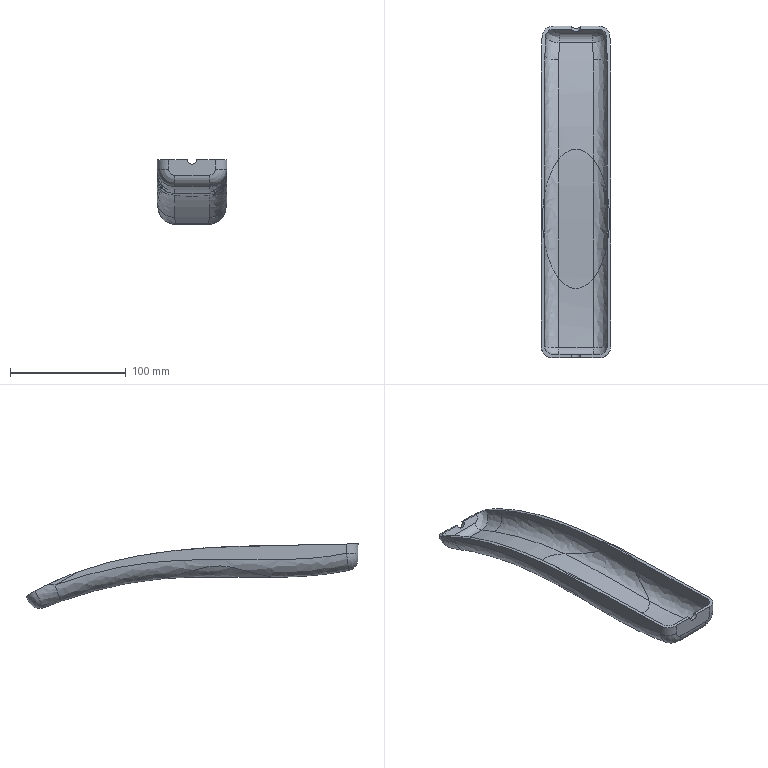Part | SolidWorks | features CompositeCurve 2 | 2 solids | 62 faces | box 60 x 286.282 x 56.047 mm | volume 79320 mm3 | spline 36 | cylinder 14 | plane 12 | commonest cylinder face diameters 14 x4 20 x4 8 x2 34 x2 40 x2